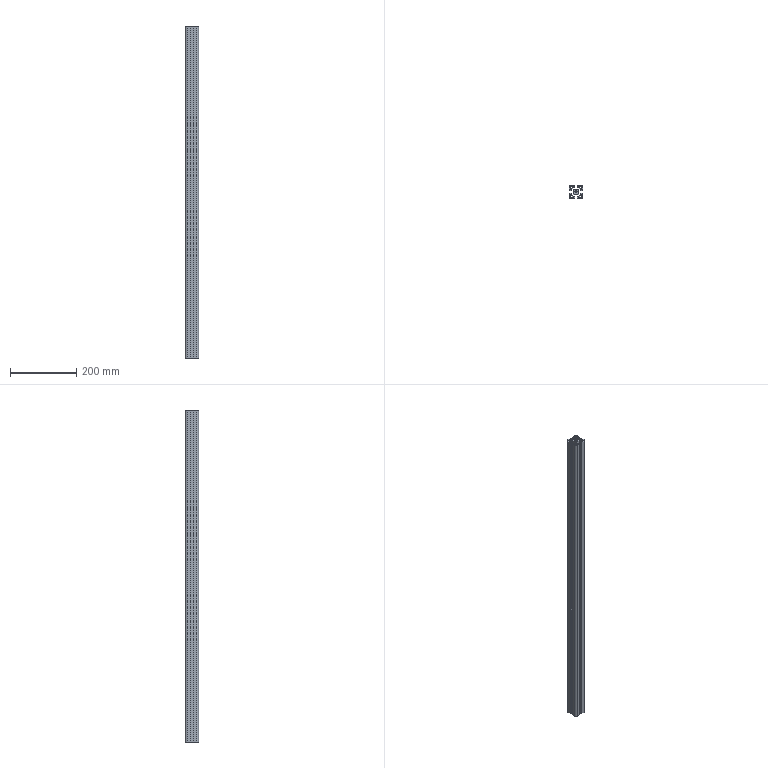Part | STEP file | 4040-1000 | 1 solid | 88 faces | box 40 x 40 x 1000 mm | volume 703947 mm3 | plane 78 | cylinder 10 | commonest cylinder face diameters 4 x4 10 x4 6.8 x2